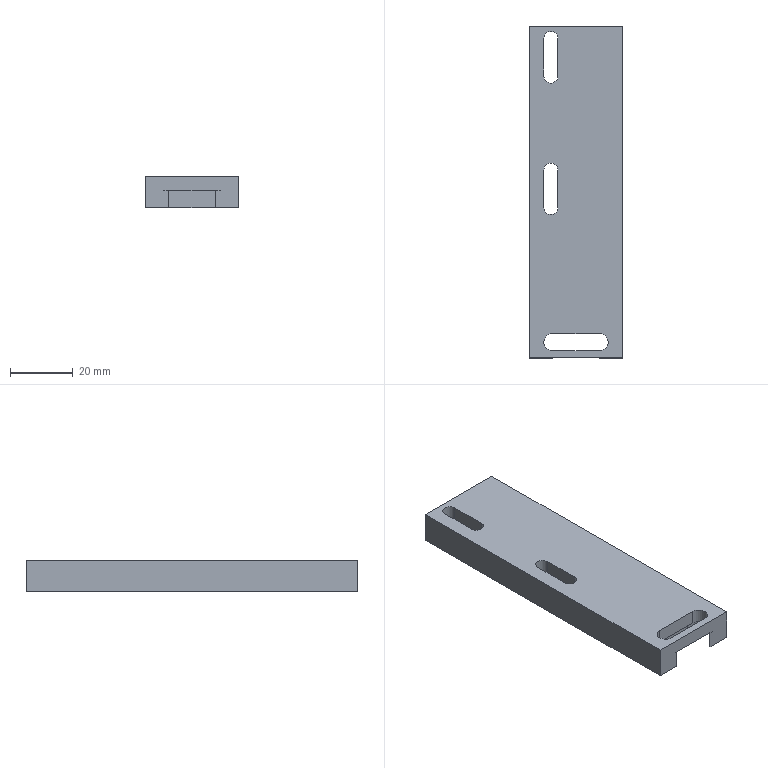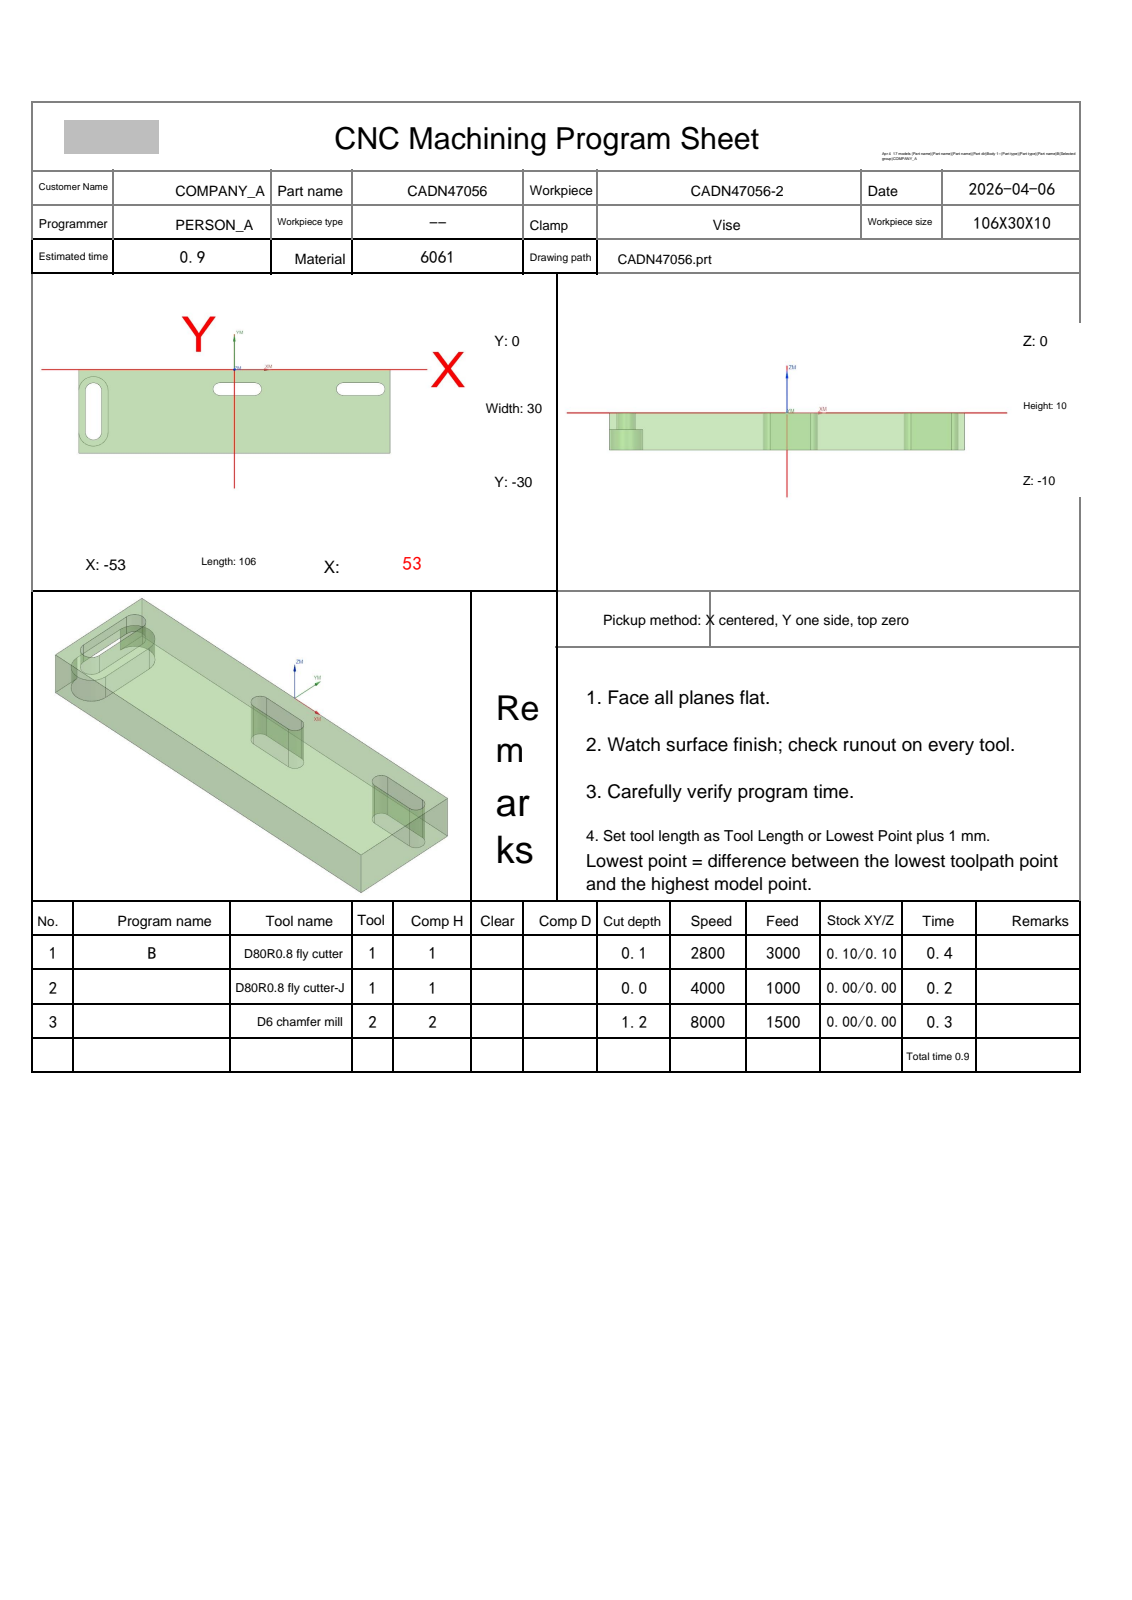NC program | NX | posted by the shop | part box 30 x 106 x 10 mm
Whole program:
%
O0001
(Machine time: 1.47 MIN)
(===Total Tool:2===)
(T1=D80R0.8 fly cutter D=80.  R=0.8  D-  H01 Z=0.    )
(T2=D6 chamfer mill   D=6.   R=0.   D-  H02 Z=-1.2  )
G80 G90 G17 G49 G40
G91 G28 Z0
M01
N1 T01 M06
(D80R0.8 fly cutter  D=80. R=0.8 H=01 ce=0.10 di=0.10)
G00 G90 G54 X-105.097 Y-15. M03 S2800
G43 H01 Z50.
M08
Z3.525
G01 Z1.525 F3000.
X-93.097
X93.097
X105.097
Z3.525
G00 X-105.097
Z3.05
G01 Z1.05
X-93.097
X93.097
X105.097
Z3.05
G00 X-105.097
Z2.575
G01 Z.575
X-93.097
X93.097
X105.097
Z2.575
G00 X-105.097
Z2.1
G01 Z.1
X-93.097
X93.097
X105.097
Z2.1
G00 Z50.
G91 G28 Z0.0
M05
M09
G91 G28 Z0.0
M01
N2 T01 M06
(D80R0.8 fly cutter-J  D=80. R=0.8 H=01 ce=0.00 di=0.00)
G00 G90 G54 X-104.999 Y-15. M03 S4000
G43 H01 Z50.
M08
Z2.
G01 Z0.0 F1000.
X-92.999
X92.999
X104.999
Z2.
G00 Z50.
G91 G28 Z0.0
M05
M09
G91 G28 Z0.0
M01
N3 T02 M06
(D6 chamfer mill  D=6. R=0. H=02 ce=0.00 di=0.00)
G00 G90 G54 X.386 Y-31.127 M03 S8000
G43 H02 Z50.
M08
Z.272
G01 Z-1.2 F1350.
G03 X.1 Y-30.927 I-1.286 J-1.532
G01 X.054 Y-30.897
X0.0 Y-30.9
X-53. F1500.
G02 X-53.9 Y-30. I0.0 J.9
G01 Y0.0
G02 X-53. Y.9 I.9 J0.0
G01 X53.
G02 X53.9 Y0.0 I0.0 J-.9
G01 Y-30.
G02 X53. Y-30.9 I-.9 J0.0
G01 X0.0
X-.054 Y-30.897
X-.1 Y-30.927
G03 X-.386 Y-31.127 I1. J-1.732
G01 Z.272
G00 Z10.
X-46.377 Y-15.386
Z.272
G01 Z-1.2 F1350.
G03 X-46.177 Y-15.1 I-1.532 J1.286
G01 X-46.147 Y-15.054
X-46.15 Y-15.
Y-7.5 F1500.
G03 X-48. Y-5.65 I-1.85 J0.0
X-49.85 Y-7.5 I0.0 J-1.85
G01 Y-22.5
G03 X-48. Y-24.35 I1.85 J0.0
X-46.15 Y-22.5 I0.0 J1.85
G01 Y-15.
X-46.147 Y-14.946
X-46.177 Y-14.9
G03 X-46.377 Y-14.614 I-1.732 J-1.
G01 Z.272
G00 Z10.
X.614 Y-8.123
Z.272
G01 Z-1.2 F1350.
G03 X.9 Y-8.323 I1.286 J1.532
G01 X.946 Y-8.353
X1. Y-8.35
X7. F1500.
G03 X8.35 Y-7. I0.0 J1.35
X7. Y-5.65 I-1.35 J0.0
G01 X-5.
G03 X-6.35 Y-7. I0.0 J-1.35
X-5. Y-8.35 I1.35 J0.0
G01 X1.
X1.054 Y-8.353
X1.1 Y-8.323
G03 X1.386 Y-8.123 I-1. J1.732
G01 Z.272
G00 Z10.
X42.614
Z.272
G01 Z-1.2 F1350.
G03 X42.9 Y-8.323 I1.286 J1.532
G01 X42.946 Y-8.353
X43. Y-8.35
X49. F1500.
G03 X50.35 Y-7. I0.0 J1.35
X49. Y-5.65 I-1.35 J0.0
G01 X37.
G03 X35.65 Y-7. I0.0 J-1.35
X37. Y-8.35 I1.35 J0.0
G01 X43.
X43.054 Y-8.353
X43.1 Y-8.323
G03 X43.386 Y-8.123 I-1. J1.732
G01 Z.272
G00 Z50.
M05
M09
G91 G28 Z0.0
G91 G28 Y0.0
M30
%